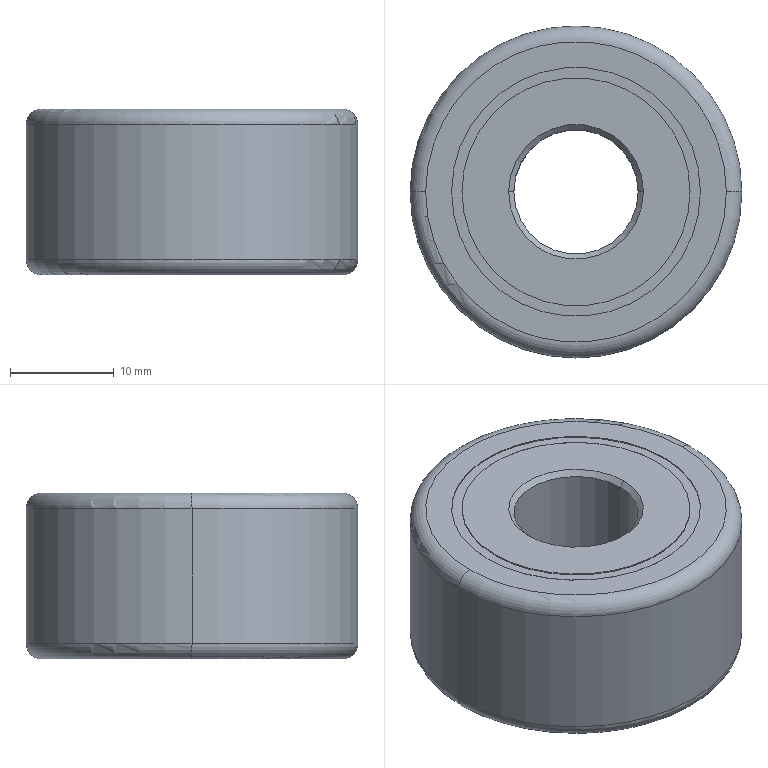Part | SolidWorks | features ICE 2, Chamfer 1, Extrusion 1, Fillet 1 | 1 solid | 20 faces | box 32 x 32 x 16 mm | volume 10946 mm3 | cylinder 8 | cone 4 | torus 4 | plane 4 | commonest cylinder face diameters 12 x2 22 x2 24 x2 32 x2
STEP:
#1=CARTESIAN_POINT('',(-6.,0.,15.5));
#2=VERTEX_POINT('',#1);
#3=CARTESIAN_POINT('',(6.,0.,15.5));
#4=VERTEX_POINT('',#3);
#5=CARTESIAN_POINT('',(0.,0.,15.5));
#6=DIRECTION('',(0.,0.,1.));
#7=DIRECTION('',(1.,0.,0.));
#8=AXIS2_PLACEMENT_3D('',#5,#6,#7);
#9=CIRCLE('',#8,6.);
#10=EDGE_CURVE('',#2,#4,#9,.T.);
#11=ORIENTED_EDGE('',*,*,#10,.F.);
#12=CARTESIAN_POINT('',(-6.5,0.,16.));
#13=VERTEX_POINT('',#12);
#14=CARTESIAN_POINT('',(-6.,0.,15.5));
#15=DIRECTION('',(-0.7071,0.,0.7071));
#16=VECTOR('',#15,1000.);
#17=LINE('',#14,#16);
#18=EDGE_CURVE('',#2,#13,#17,.T.);
#19=ORIENTED_EDGE('',*,*,#18,.T.);
#20=CARTESIAN_POINT('',(6.5,0.,16.));
#21=VERTEX_POINT('',#20);
#22=CARTESIAN_POINT('',(0.,0.,16.));
#23=DIRECTION('',(0.,0.,-1.));
#24=DIRECTION('',(1.,0.,0.));
#25=AXIS2_PLACEMENT_3D('',#22,#23,#24);
#26=CIRCLE('',#25,6.5);
#27=EDGE_CURVE('',#21,#13,#26,.T.);
#28=ORIENTED_EDGE('',*,*,#27,.F.);
#29=CARTESIAN_POINT('',(6.,0.,15.5));
#30=DIRECTION('',(0.7071,0.,0.7071));
#31=VECTOR('',#30,1000.);
#32=LINE('',#29,#31);
#33=EDGE_CURVE('',#4,#21,#32,.T.);
#34=ORIENTED_EDGE('',*,*,#33,.F.);
#35=EDGE_LOOP('',(#11,#19,#28,#34));
#36=FACE_OUTER_BOUND('',#35,.T.);
#37=CARTESIAN_POINT('',(0.,0.,15.5));
#38=DIRECTION('',(0.,0.,1.));
#39=DIRECTION('',(1.,0.,0.));
#40=AXIS2_PLACEMENT_3D('',#37,#38,#39);
#41=CONICAL_SURFACE('',#40,6.,0.7854);
#42=ADVANCED_FACE('',(#36),#41,.F.);
#43=CARTESIAN_POINT('',(6.,0.,0.5));
#44=VERTEX_POINT('',#43);
#45=CARTESIAN_POINT('',(-6.,0.,0.5));
#46=VERTEX_POINT('',#45);
#47=CARTESIAN_POINT('',(0.,0.,0.5));
#48=DIRECTION('',(0.,0.,-1.));
#49=DIRECTION('',(1.,0.,0.));
#50=AXIS2_PLACEMENT_3D('',#47,#48,#49);
#51=CIRCLE('',#50,6.);
#52=EDGE_CURVE('',#44,#46,#51,.T.);
#53=ORIENTED_EDGE('',*,*,#52,.F.);
#54=CARTESIAN_POINT('',(6.5,0.,0.));
#55=VERTEX_POINT('',#54);
#56=CARTESIAN_POINT('',(6.5,0.,0.));
#57=DIRECTION('',(0.7071,0.,-0.7071));
#58=VECTOR('',#57,1000.);
#59=LINE('',#56,#58);
#60=EDGE_CURVE('',#44,#55,#59,.T.);
#61=ORIENTED_EDGE('',*,*,#60,.T.);
#62=CARTESIAN_POINT('',(-6.5,0.,0.));
#63=VERTEX_POINT('',#62);
#64=CARTESIAN_POINT('',(0.,0.,0.));
#65=DIRECTION('',(0.,0.,1.));
#66=DIRECTION('',(1.,0.,0.));
#67=AXIS2_PLACEMENT_3D('',#64,#65,#66);
#68=CIRCLE('',#67,6.5);
#69=EDGE_CURVE('',#63,#55,#68,.T.);
#70=ORIENTED_EDGE('',*,*,#69,.F.);
#71=CARTESIAN_POINT('',(-6.5,0.,0.));
#72=DIRECTION('',(-0.7071,0.,-0.7071));
#73=VECTOR('',#72,1000.);
#74=LINE('',#71,#73);
#75=EDGE_CURVE('',#46,#63,#74,.T.);
#76=ORIENTED_EDGE('',*,*,#75,.F.);
#77=EDGE_LOOP('',(#53,#61,#70,#76));
#78=FACE_OUTER_BOUND('',#77,.T.);
#79=CARTESIAN_POINT('',(0.,0.,0.));
#80=DIRECTION('',(0.,0.,-1.));
#81=DIRECTION('',(-1.,0.,0.));
#82=AXIS2_PLACEMENT_3D('',#79,#80,#81);
#83=CONICAL_SURFACE('',#82,6.5,0.7854);
#84=ADVANCED_FACE('',(#78),#83,.F.);
#85=CARTESIAN_POINT('',(-16.,0.,14.5));
#86=VERTEX_POINT('',#85);
#87=CARTESIAN_POINT('',(16.,0.,14.5));
#88=VERTEX_POINT('',#87);
#89=CARTESIAN_POINT('',(0.,0.,14.5));
#90=DIRECTION('',(0.,0.,-1.));
#91=DIRECTION('',(1.,0.,0.));
#92=AXIS2_PLACEMENT_3D('',#89,#90,#91);
#93=CIRCLE('',#92,16.);
#94=EDGE_CURVE('',#86,#88,#93,.T.);
#95=ORIENTED_EDGE('',*,*,#94,.F.);
#96=CARTESIAN_POINT('',(-14.5,0.,16.));
#97=VERTEX_POINT('',#96);
#98=CARTESIAN_POINT('',(-14.5,0.,14.5));
#99=DIRECTION('',(0.,1.,0.));
#100=DIRECTION('',(-1.,0.,0.));
#101=AXIS2_PLACEMENT_3D('',#98,#99,#100);
#102=CIRCLE('',#101,1.5);
#103=EDGE_CURVE('',#86,#97,#102,.T.);
#104=ORIENTED_EDGE('',*,*,#103,.T.);
#105=CARTESIAN_POINT('',(14.5,0.,16.));
#106=VERTEX_POINT('',#105);
#107=CARTESIAN_POINT('',(0.,0.,16.));
#108=DIRECTION('',(0.,0.,1.));
#109=DIRECTION('',(1.,0.,0.));
#110=AXIS2_PLACEMENT_3D('',#107,#108,#109);
#111=CIRCLE('',#110,14.5);
#112=EDGE_CURVE('',#106,#97,#111,.T.);
#113=ORIENTED_EDGE('',*,*,#112,.F.);
#114=CARTESIAN_POINT('',(14.5,0.,14.5));
#115=DIRECTION('',(0.,-1.,0.));
#116=DIRECTION('',(0.,0.,-1.));
#117=AXIS2_PLACEMENT_3D('',#114,#115,#116);
#118=CIRCLE('',#117,1.5);
#119=EDGE_CURVE('',#88,#106,#118,.T.);
#120=ORIENTED_EDGE('',*,*,#119,.F.);
#121=EDGE_LOOP('',(#95,#104,#113,#120));
#122=FACE_OUTER_BOUND('',#121,.T.);
#123=CARTESIAN_POINT('',(0.,0.,14.5));
#124=DIRECTION('',(0.,0.,1.));
#125=DIRECTION('',(1.,0.,0.));
#126=AXIS2_PLACEMENT_3D('',#123,#124,#125);
#127=TOROIDAL_SURFACE('',#126,14.5,1.5);
#128=ADVANCED_FACE('',(#122),#127,.T.);
#129=CARTESIAN_POINT('',(-14.5,0.,0.));
#130=VERTEX_POINT('',#129);
#131=CARTESIAN_POINT('',(14.5,0.,0.));
#132=VERTEX_POINT('',#131);
#133=CARTESIAN_POINT('',(0.,0.,0.));
#134=DIRECTION('',(0.,0.,-1.));
#135=DIRECTION('',(1.,0.,0.));
#136=AXIS2_PLACEMENT_3D('',#133,#134,#135);
#137=CIRCLE('',#136,14.5);
#138=EDGE_CURVE('',#130,#132,#137,.T.);
#139=ORIENTED_EDGE('',*,*,#138,.F.);
#140=CARTESIAN_POINT('',(-16.,0.,1.5));
#141=VERTEX_POINT('',#140);
#142=CARTESIAN_POINT('',(-14.5,0.,1.5));
#143=DIRECTION('',(0.,1.,0.));
#144=DIRECTION('',(-1.,0.,0.));
#145=AXIS2_PLACEMENT_3D('',#142,#143,#144);
#146=CIRCLE('',#145,1.5);
#147=EDGE_CURVE('',#130,#141,#146,.T.);
#148=ORIENTED_EDGE('',*,*,#147,.T.);
#149=CARTESIAN_POINT('',(16.,0.,1.5));
#150=VERTEX_POINT('',#149);
#151=CARTESIAN_POINT('',(0.,0.,1.5));
#152=DIRECTION('',(0.,0.,1.));
#153=DIRECTION('',(1.,0.,0.));
#154=AXIS2_PLACEMENT_3D('',#151,#152,#153);
#155=CIRCLE('',#154,16.);
#156=EDGE_CURVE('',#150,#141,#155,.T.);
#157=ORIENTED_EDGE('',*,*,#156,.F.);
#158=CARTESIAN_POINT('',(14.5,0.,1.5));
#159=DIRECTION('',(0.,-1.,0.));
#160=DIRECTION('',(0.,0.,-1.));
#161=AXIS2_PLACEMENT_3D('',#158,#159,#160);
#162=CIRCLE('',#161,1.5);
#163=EDGE_CURVE('',#132,#150,#162,.T.);
#164=ORIENTED_EDGE('',*,*,#163,.F.);
#165=EDGE_LOOP('',(#139,#148,#157,#164));
#166=FACE_OUTER_BOUND('',#165,.T.);
#167=CARTESIAN_POINT('',(0.,0.,1.5));
#168=DIRECTION('',(0.,0.,1.));
#169=DIRECTION('',(1.,0.,0.));
#170=AXIS2_PLACEMENT_3D('',#167,#168,#169);
#171=TOROIDAL_SURFACE('',#170,14.5,1.5);
#172=ADVANCED_FACE('',(#166),#171,.T.);
#173=CARTESIAN_POINT('',(11.,0.,15.9));
#174=VERTEX_POINT('',#173);
#175=CARTESIAN_POINT('',(-11.,0.,15.9));
#176=VERTEX_POINT('',#175);
#177=CARTESIAN_POINT('',(0.,0.,15.9));
#178=DIRECTION('',(0.,0.,1.));
#179=DIRECTION('',(1.,0.,0.));
#180=AXIS2_PLACEMENT_3D('',#177,#178,#179);
#181=CIRCLE('',#180,11.);
#182=EDGE_CURVE('',#174,#176,#181,.T.);
#183=ORIENTED_EDGE('',*,*,#182,.T.);
#184=CARTESIAN_POINT('',(-11.,0.,16.));
#185=VERTEX_POINT('',#184);
#186=CARTESIAN_POINT('',(-11.,0.,15.9));
#187=DIRECTION('',(0.,0.,1.));
#188=VECTOR('',#187,1000.);
#189=LINE('',#186,#188);
#190=EDGE_CURVE('',#176,#185,#189,.T.);
#191=ORIENTED_EDGE('',*,*,#190,.T.);
#192=CARTESIAN_POINT('',(11.,0.,16.));
#193=VERTEX_POINT('',#192);
#194=CARTESIAN_POINT('',(0.,0.,16.));
#195=DIRECTION('',(0.,0.,1.));
#196=DIRECTION('',(1.,0.,0.));
#197=AXIS2_PLACEMENT_3D('',#194,#195,#196);
#198=CIRCLE('',#197,11.);
#199=EDGE_CURVE('',#193,#185,#198,.T.);
#200=ORIENTED_EDGE('',*,*,#199,.F.);
#201=CARTESIAN_POINT('',(11.,0.,15.9));
#202=DIRECTION('',(0.,0.,1.));
#203=VECTOR('',#202,1000.);
#204=LINE('',#201,#203);
#205=EDGE_CURVE('',#174,#193,#204,.T.);
#206=ORIENTED_EDGE('',*,*,#205,.F.);
#207=EDGE_LOOP('',(#183,#191,#200,#206));
#208=FACE_OUTER_BOUND('',#207,.T.);
#209=CARTESIAN_POINT('',(0.,0.,15.9));
#210=DIRECTION('',(0.,0.,1.));
#211=DIRECTION('',(1.,0.,0.));
#212=AXIS2_PLACEMENT_3D('',#209,#210,#211);
#213=CYLINDRICAL_SURFACE('',#212,11.);
#214=ADVANCED_FACE('',(#208),#213,.T.);
#215=CARTESIAN_POINT('',(-12.,0.,15.9));
#216=VERTEX_POINT('',#215);
#217=CARTESIAN_POINT('',(12.,0.,15.9));
#218=VERTEX_POINT('',#217);
#219=CARTESIAN_POINT('',(0.,0.,15.9));
#220=DIRECTION('',(0.,0.,1.));
#221=DIRECTION('',(1.,0.,0.));
#222=AXIS2_PLACEMENT_3D('',#219,#220,#221);
#223=CIRCLE('',#222,12.);
#224=EDGE_CURVE('',#216,#218,#223,.T.);
#225=ORIENTED_EDGE('',*,*,#224,.F.);
#226=CARTESIAN_POINT('',(-12.,0.,16.));
#227=VERTEX_POINT('',#226);
#228=CARTESIAN_POINT('',(-12.,0.,15.9));
#229=DIRECTION('',(0.,0.,1.));
#230=VECTOR('',#229,1000.);
#231=LINE('',#228,#230);
#232=EDGE_CURVE('',#216,#227,#231,.T.);
#233=ORIENTED_EDGE('',*,*,#232,.T.);
#234=CARTESIAN_POINT('',(12.,0.,16.));
#235=VERTEX_POINT('',#234);
#236=CARTESIAN_POINT('',(0.,0.,16.));
#237=DIRECTION('',(0.,0.,1.));
#238=DIRECTION('',(1.,0.,0.));
#239=AXIS2_PLACEMENT_3D('',#236,#237,#238);
#240=CIRCLE('',#239,12.);
#241=EDGE_CURVE('',#227,#235,#240,.T.);
#242=ORIENTED_EDGE('',*,*,#241,.T.);
#243=CARTESIAN_POINT('',(12.,0.,15.9));
#244=DIRECTION('',(0.,0.,1.));
#245=VECTOR('',#244,1000.);
#246=LINE('',#243,#245);
#247=EDGE_CURVE('',#218,#235,#246,.T.);
#248=ORIENTED_EDGE('',*,*,#247,.F.);
#249=EDGE_LOOP('',(#225,#233,#242,#248));
#250=FACE_OUTER_BOUND('',#249,.T.);
#251=CARTESIAN_POINT('',(0.,0.,15.9));
#252=DIRECTION('',(0.,0.,1.));
#253=DIRECTION('',(1.,0.,0.));
#254=AXIS2_PLACEMENT_3D('',#251,#252,#253);
#255=CYLINDRICAL_SURFACE('',#254,12.);
#256=ADVANCED_FACE('',(#250),#255,.F.);
#257=ORIENTED_EDGE('',*,*,#52,.T.);
#258=CARTESIAN_POINT('',(-6.,0.,0.));
#259=DIRECTION('',(0.,0.,1.));
#260=VECTOR('',#259,1000.);
#261=LINE('',#258,#260);
#262=EDGE_CURVE('',#46,#2,#261,.T.);
#263=ORIENTED_EDGE('',*,*,#262,.T.);
#264=ORIENTED_EDGE('',*,*,#10,.T.);
#265=CARTESIAN_POINT('',(6.,0.,0.));
#266=DIRECTION('',(0.,0.,1.));
#267=VECTOR('',#266,1000.);
#268=LINE('',#265,#267);
#269=EDGE_CURVE('',#44,#4,#268,.T.);
#270=ORIENTED_EDGE('',*,*,#269,.F.);
#271=EDGE_LOOP('',(#257,#263,#264,#270));
#272=FACE_OUTER_BOUND('',#271,.T.);
#273=CARTESIAN_POINT('',(0.,0.,0.));
#274=DIRECTION('',(0.,0.,1.));
#275=DIRECTION('',(1.,0.,0.));
#276=AXIS2_PLACEMENT_3D('',#273,#274,#275);
#277=CYLINDRICAL_SURFACE('',#276,6.);
#278=ADVANCED_FACE('',(#272),#277,.F.);
#279=ORIENTED_EDGE('',*,*,#94,.T.);
#280=CARTESIAN_POINT('',(16.,0.,16.));
#281=DIRECTION('',(0.,0.,-1.));
#282=VECTOR('',#281,1000.);
#283=LINE('',#280,#282);
#284=EDGE_CURVE('',#88,#150,#283,.T.);
#285=ORIENTED_EDGE('',*,*,#284,.T.);
#286=ORIENTED_EDGE('',*,*,#156,.T.);
#287=CARTESIAN_POINT('',(-16.,0.,16.));
#288=DIRECTION('',(0.,0.,-1.));
#289=VECTOR('',#288,1000.);
#290=LINE('',#287,#289);
#291=EDGE_CURVE('',#86,#141,#290,.T.);
#292=ORIENTED_EDGE('',*,*,#291,.F.);
#293=EDGE_LOOP('',(#279,#285,#286,#292));
#294=FACE_OUTER_BOUND('',#293,.T.);
#295=CARTESIAN_POINT('',(0.,0.,16.));
#296=DIRECTION('',(0.,0.,-1.));
#297=DIRECTION('',(-1.,0.,0.));
#298=AXIS2_PLACEMENT_3D('',#295,#296,#297);
#299=CYLINDRICAL_SURFACE('',#298,16.);
#300=ADVANCED_FACE('',(#294),#299,.T.);
#301=ORIENTED_EDGE('',*,*,#27,.T.);
#302=CARTESIAN_POINT('',(0.,0.,16.));
#303=DIRECTION('',(0.,0.,-1.));
#304=DIRECTION('',(1.,0.,0.));
#305=AXIS2_PLACEMENT_3D('',#302,#303,#304);
#306=CIRCLE('',#305,6.5);
#307=EDGE_CURVE('',#13,#21,#306,.T.);
#308=ORIENTED_EDGE('',*,*,#307,.T.);
#309=EDGE_LOOP('',(#301,#308));
#310=FACE_BOUND('',#309,.T.);
#311=ORIENTED_EDGE('',*,*,#199,.T.);
#312=CARTESIAN_POINT('',(0.,0.,16.));
#313=DIRECTION('',(0.,0.,1.));
#314=DIRECTION('',(1.,0.,0.));
#315=AXIS2_PLACEMENT_3D('',#312,#313,#314);
#316=CIRCLE('',#315,11.);
#317=EDGE_CURVE('',#185,#193,#316,.T.);
#318=ORIENTED_EDGE('',*,*,#317,.T.);
#319=EDGE_LOOP('',(#311,#318));
#320=FACE_OUTER_BOUND('',#319,.T.);
#321=CARTESIAN_POINT('',(0.,0.,16.));
#322=DIRECTION('',(0.,0.,1.));
#323=DIRECTION('',(1.,0.,0.));
#324=AXIS2_PLACEMENT_3D('',#321,#322,#323);
#325=PLANE('',#324);
#326=ADVANCED_FACE('',(#310,#320),#325,.T.);
#327=ORIENTED_EDGE('',*,*,#284,.F.);
#328=CARTESIAN_POINT('',(0.,0.,14.5));
#329=DIRECTION('',(0.,0.,-1.));
#330=DIRECTION('',(1.,0.,0.));
#331=AXIS2_PLACEMENT_3D('',#328,#329,#330);
#332=CIRCLE('',#331,16.);
#333=EDGE_CURVE('',#88,#86,#332,.T.);
#334=ORIENTED_EDGE('',*,*,#333,.T.);
#335=ORIENTED_EDGE('',*,*,#291,.T.);
#336=CARTESIAN_POINT('',(0.,0.,1.5));
#337=DIRECTION('',(0.,0.,1.));
#338=DIRECTION('',(1.,0.,0.));
#339=AXIS2_PLACEMENT_3D('',#336,#337,#338);
#340=CIRCLE('',#339,16.);
#341=EDGE_CURVE('',#141,#150,#340,.T.);
#342=ORIENTED_EDGE('',*,*,#341,.T.);
#343=EDGE_LOOP('',(#327,#334,#335,#342));
#344=FACE_OUTER_BOUND('',#343,.T.);
#345=CARTESIAN_POINT('',(0.,0.,16.));
#346=DIRECTION('',(0.,0.,-1.));
#347=DIRECTION('',(-1.,0.,0.));
#348=AXIS2_PLACEMENT_3D('',#345,#346,#347);
#349=CYLINDRICAL_SURFACE('',#348,16.);
#350=ADVANCED_FACE('',(#344),#349,.T.);
#351=ORIENTED_EDGE('',*,*,#112,.T.);
#352=CARTESIAN_POINT('',(0.,0.,16.));
#353=DIRECTION('',(0.,0.,1.));
#354=DIRECTION('',(1.,0.,0.));
#355=AXIS2_PLACEMENT_3D('',#352,#353,#354);
#356=CIRCLE('',#355,14.5);
#357=EDGE_CURVE('',#97,#106,#356,.T.);
#358=ORIENTED_EDGE('',*,*,#357,.T.);
#359=EDGE_LOOP('',(#351,#358));
#360=FACE_OUTER_BOUND('',#359,.T.);
#361=CARTESIAN_POINT('',(0.,0.,16.));
#362=DIRECTION('',(0.,0.,1.));
#363=DIRECTION('',(1.,0.,0.));
#364=AXIS2_PLACEMENT_3D('',#361,#362,#363);
#365=CIRCLE('',#364,12.);
#366=EDGE_CURVE('',#235,#227,#365,.T.);
#367=ORIENTED_EDGE('',*,*,#366,.F.);
#368=ORIENTED_EDGE('',*,*,#241,.F.);
#369=EDGE_LOOP('',(#367,#368));
#370=FACE_BOUND('',#369,.T.);
#371=CARTESIAN_POINT('',(0.,0.,16.));
#372=DIRECTION('',(0.,0.,1.));
#373=DIRECTION('',(1.,0.,0.));
#374=AXIS2_PLACEMENT_3D('',#371,#372,#373);
#375=PLANE('',#374);
#376=ADVANCED_FACE('',(#360,#370),#375,.T.);
#377=ORIENTED_EDGE('',*,*,#69,.T.);
#378=CARTESIAN_POINT('',(0.,0.,0.));
#379=DIRECTION('',(0.,0.,1.));
#380=DIRECTION('',(1.,0.,0.));
#381=AXIS2_PLACEMENT_3D('',#378,#379,#380);
#382=CIRCLE('',#381,6.5);
#383=EDGE_CURVE('',#55,#63,#382,.T.);
#384=ORIENTED_EDGE('',*,*,#383,.T.);
#385=EDGE_LOOP('',(#377,#384));
#386=FACE_BOUND('',#385,.T.);
#387=CARTESIAN_POINT('',(0.,0.,0.));
#388=DIRECTION('',(0.,0.,-1.));
#389=DIRECTION('',(1.,0.,0.));
#390=AXIS2_PLACEMENT_3D('',#387,#388,#389);
#391=CIRCLE('',#390,14.5);
#392=EDGE_CURVE('',#132,#130,#391,.T.);
#393=ORIENTED_EDGE('',*,*,#392,.T.);
#394=ORIENTED_EDGE('',*,*,#138,.T.);
#395=EDGE_LOOP('',(#393,#394));
#396=FACE_OUTER_BOUND('',#395,.T.);
#397=CARTESIAN_POINT('',(0.,0.,0.));
#398=DIRECTION('',(0.,0.,1.));
#399=DIRECTION('',(1.,0.,0.));
#400=AXIS2_PLACEMENT_3D('',#397,#398,#399);
#401=PLANE('',#400);
#402=ADVANCED_FACE('',(#386,#396),#401,.F.);
#403=ORIENTED_EDGE('',*,*,#262,.F.);
#404=CARTESIAN_POINT('',(0.,0.,0.5));
#405=DIRECTION('',(0.,0.,-1.));
#406=DIRECTION('',(1.,0.,0.));
#407=AXIS2_PLACEMENT_3D('',#404,#405,#406);
#408=CIRCLE('',#407,6.);
#409=EDGE_CURVE('',#46,#44,#408,.T.);
#410=ORIENTED_EDGE('',*,*,#409,.T.);
#411=ORIENTED_EDGE('',*,*,#269,.T.);
#412=CARTESIAN_POINT('',(0.,0.,15.5));
#413=DIRECTION('',(0.,0.,1.));
#414=DIRECTION('',(1.,0.,0.));
#415=AXIS2_PLACEMENT_3D('',#412,#413,#414);
#416=CIRCLE('',#415,6.);
#417=EDGE_CURVE('',#4,#2,#416,.T.);
#418=ORIENTED_EDGE('',*,*,#417,.T.);
#419=EDGE_LOOP('',(#403,#410,#411,#418));
#420=FACE_OUTER_BOUND('',#419,.T.);
#421=CARTESIAN_POINT('',(0.,0.,0.));
#422=DIRECTION('',(0.,0.,1.));
#423=DIRECTION('',(1.,0.,0.));
#424=AXIS2_PLACEMENT_3D('',#421,#422,#423);
#425=CYLINDRICAL_SURFACE('',#424,6.);
#426=ADVANCED_FACE('',(#420),#425,.F.);
#427=ORIENTED_EDGE('',*,*,#232,.F.);
#428=CARTESIAN_POINT('',(0.,0.,15.9));
#429=DIRECTION('',(0.,0.,1.));
#430=DIRECTION('',(1.,0.,0.));
#431=AXIS2_PLACEMENT_3D('',#428,#429,#430);
#432=CIRCLE('',#431,12.);
#433=EDGE_CURVE('',#218,#216,#432,.T.);
#434=ORIENTED_EDGE('',*,*,#433,.F.);
#435=ORIENTED_EDGE('',*,*,#247,.T.);
#436=ORIENTED_EDGE('',*,*,#366,.T.);
#437=EDGE_LOOP('',(#427,#434,#435,#436));
#438=FACE_OUTER_BOUND('',#437,.T.);
#439=CARTESIAN_POINT('',(0.,0.,15.9));
#440=DIRECTION('',(0.,0.,1.));
#441=DIRECTION('',(1.,0.,0.));
#442=AXIS2_PLACEMENT_3D('',#439,#440,#441);
#443=CYLINDRICAL_SURFACE('',#442,12.);
#444=ADVANCED_FACE('',(#438),#443,.F.);
#445=ORIENTED_EDGE('',*,*,#182,.F.);
#446=CARTESIAN_POINT('',(0.,0.,15.9));
#447=DIRECTION('',(0.,0.,1.));
#448=DIRECTION('',(1.,0.,0.));
#449=AXIS2_PLACEMENT_3D('',#446,#447,#448);
#450=CIRCLE('',#449,11.);
#451=EDGE_CURVE('',#176,#174,#450,.T.);
#452=ORIENTED_EDGE('',*,*,#451,.F.);
#453=EDGE_LOOP('',(#445,#452));
#454=FACE_BOUND('',#453,.T.);
#455=ORIENTED_EDGE('',*,*,#433,.T.);
#456=ORIENTED_EDGE('',*,*,#224,.T.);
#457=EDGE_LOOP('',(#455,#456));
#458=FACE_OUTER_BOUND('',#457,.T.);
#459=CARTESIAN_POINT('',(0.,0.,15.9));
#460=DIRECTION('',(0.,0.,1.));
#461=DIRECTION('',(1.,0.,0.));
#462=AXIS2_PLACEMENT_3D('',#459,#460,#461);
#463=PLANE('',#462);
#464=ADVANCED_FACE('',(#454,#458),#463,.T.);
#465=ORIENTED_EDGE('',*,*,#190,.F.);
#466=ORIENTED_EDGE('',*,*,#451,.T.);
#467=ORIENTED_EDGE('',*,*,#205,.T.);
#468=ORIENTED_EDGE('',*,*,#317,.F.);
#469=EDGE_LOOP('',(#465,#466,#467,#468));
#470=FACE_OUTER_BOUND('',#469,.T.);
#471=CARTESIAN_POINT('',(0.,0.,15.9));
#472=DIRECTION('',(0.,0.,1.));
#473=DIRECTION('',(1.,0.,0.));
#474=AXIS2_PLACEMENT_3D('',#471,#472,#473);
#475=CYLINDRICAL_SURFACE('',#474,11.);
#476=ADVANCED_FACE('',(#470),#475,.T.);
#477=ORIENTED_EDGE('',*,*,#147,.F.);
#478=ORIENTED_EDGE('',*,*,#392,.F.);
#479=ORIENTED_EDGE('',*,*,#163,.T.);
#480=ORIENTED_EDGE('',*,*,#341,.F.);
#481=EDGE_LOOP('',(#477,#478,#479,#480));
#482=FACE_OUTER_BOUND('',#481,.T.);
#483=CARTESIAN_POINT('',(0.,0.,1.5));
#484=DIRECTION('',(0.,0.,1.));
#485=DIRECTION('',(1.,0.,0.));
#486=AXIS2_PLACEMENT_3D('',#483,#484,#485);
#487=TOROIDAL_SURFACE('',#486,14.5,1.5);
#488=ADVANCED_FACE('',(#482),#487,.T.);
#489=ORIENTED_EDGE('',*,*,#103,.F.);
#490=ORIENTED_EDGE('',*,*,#333,.F.);
#491=ORIENTED_EDGE('',*,*,#119,.T.);
#492=ORIENTED_EDGE('',*,*,#357,.F.);
#493=EDGE_LOOP('',(#489,#490,#491,#492));
#494=FACE_OUTER_BOUND('',#493,.T.);
#495=CARTESIAN_POINT('',(0.,0.,14.5));
#496=DIRECTION('',(0.,0.,1.));
#497=DIRECTION('',(1.,0.,0.));
#498=AXIS2_PLACEMENT_3D('',#495,#496,#497);
#499=TOROIDAL_SURFACE('',#498,14.5,1.5);
#500=ADVANCED_FACE('',(#494),#499,.T.);
#501=ORIENTED_EDGE('',*,*,#60,.F.);
#502=ORIENTED_EDGE('',*,*,#409,.F.);
#503=ORIENTED_EDGE('',*,*,#75,.T.);
#504=ORIENTED_EDGE('',*,*,#383,.F.);
#505=EDGE_LOOP('',(#501,#502,#503,#504));
#506=FACE_OUTER_BOUND('',#505,.T.);
#507=CARTESIAN_POINT('',(0.,0.,0.));
#508=DIRECTION('',(0.,0.,-1.));
#509=DIRECTION('',(-1.,0.,0.));
#510=AXIS2_PLACEMENT_3D('',#507,#508,#509);
#511=CONICAL_SURFACE('',#510,6.5,0.7854);
#512=ADVANCED_FACE('',(#506),#511,.F.);
#513=ORIENTED_EDGE('',*,*,#18,.F.);
#514=ORIENTED_EDGE('',*,*,#417,.F.);
#515=ORIENTED_EDGE('',*,*,#33,.T.);
#516=ORIENTED_EDGE('',*,*,#307,.F.);
#517=EDGE_LOOP('',(#513,#514,#515,#516));
#518=FACE_OUTER_BOUND('',#517,.T.);
#519=CARTESIAN_POINT('',(0.,0.,15.5));
#520=DIRECTION('',(0.,0.,1.));
#521=DIRECTION('',(1.,0.,0.));
#522=AXIS2_PLACEMENT_3D('',#519,#520,#521);
#523=CONICAL_SURFACE('',#522,6.,0.7854);
#524=ADVANCED_FACE('',(#518),#523,.F.);
#525=CLOSED_SHELL('',(#42,#84,#128,#172,#214,#256,#278,#300,#326,#350,#376,#402,#426,#444,#464,#476,#488,#500,#512,#524));
#526=MANIFOLD_SOLID_BREP('',#525);
#527=CARTESIAN_POINT('',(0.,0.,0.));
#528=DIRECTION('',(0.,0.,1.));
#529=DIRECTION('',(1.,0.,0.));
#530=AXIS2_PLACEMENT_3D('',#527,#528,#529);
#531=(LENGTH_UNIT()NAMED_UNIT(*)SI_UNIT(.MILLI.,.METRE.));
#532=UNCERTAINTY_MEASURE_WITH_UNIT(LENGTH_MEASURE(0.00001),#531,'','');
#533=(NAMED_UNIT(*)PLANE_ANGLE_UNIT()SI_UNIT($,.RADIAN.));
#534=(NAMED_UNIT(*)SI_UNIT($,.STERADIAN.)SOLID_ANGLE_UNIT());
#535=(GEOMETRIC_REPRESENTATION_CONTEXT(3)GLOBAL_UNCERTAINTY_ASSIGNED_CONTEXT((#532))GLOBAL_UNIT_ASSIGNED_CONTEXT((#531,#533,#534))REPRESENTATION_CONTEXT('',''));
#536=ADVANCED_BREP_SHAPE_REPRESENTATION('',(#526,#530),#535);